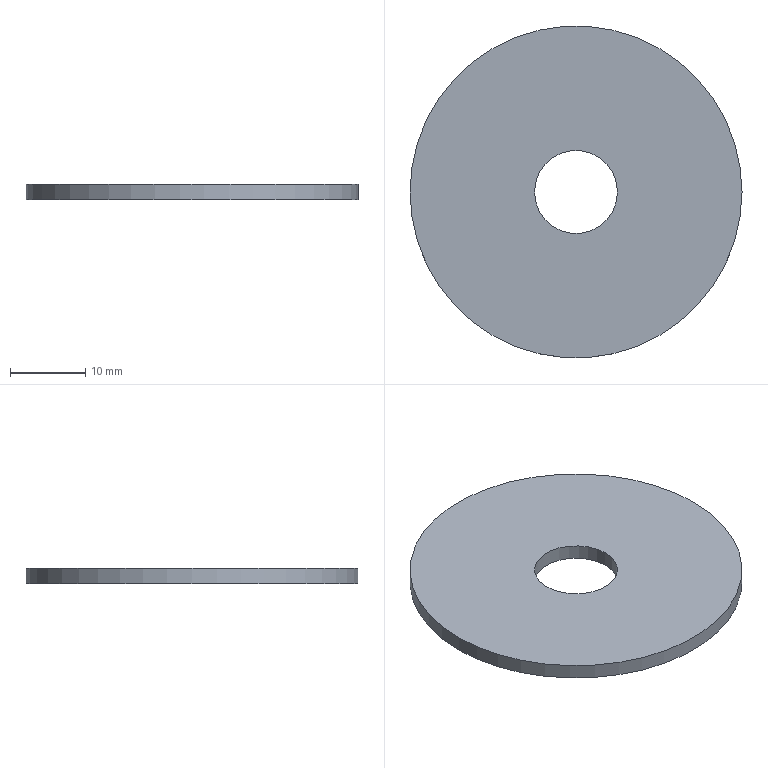Part | NX | features CYLINDER 1, DATUM_CSYS 1, HOLE PACKAGE 1, SIMPLE HOLE 1 | 1 solid | 4 faces | box 44 x 44 x 2 mm | volume 2851 mm3 | plane 2 | cylinder 2 | commonest cylinder face diameters 11 x1 44 x1
STEP:
#1=CARTESIAN_POINT('',(5.5,0.,2.));
#2=VERTEX_POINT('',#1);
#3=CARTESIAN_POINT('',(0.,0.,2.));
#4=DIRECTION('',(0.,0.,1.));
#5=DIRECTION('',(1.,0.,0.));
#6=AXIS2_PLACEMENT_3D('',#3,#4,#5);
#7=CIRCLE('',#6,5.5);
#8=EDGE_CURVE('',#2,#2,#7,.T.);
#9=ORIENTED_EDGE('',*,*,#8,.F.);
#10=EDGE_LOOP('',(#9));
#11=FACE_BOUND('',#10,.T.);
#12=CARTESIAN_POINT('',(-22.,0.,2.));
#13=VERTEX_POINT('',#12);
#14=CARTESIAN_POINT('',(0.,0.,2.));
#15=DIRECTION('',(0.,0.,-1.));
#16=DIRECTION('',(-1.,0.,0.));
#17=AXIS2_PLACEMENT_3D('',#14,#15,#16);
#18=CIRCLE('',#17,22.);
#19=EDGE_CURVE('',#13,#13,#18,.T.);
#20=ORIENTED_EDGE('',*,*,#19,.F.);
#21=EDGE_LOOP('',(#20));
#22=FACE_BOUND('',#21,.T.);
#23=CARTESIAN_POINT('',(0.,0.,2.));
#24=DIRECTION('',(0.,0.,1.));
#25=DIRECTION('',(1.,0.,0.));
#26=AXIS2_PLACEMENT_3D('',#23,#24,#25);
#27=PLANE('',#26);
#28=ADVANCED_FACE('',(#11,#22),#27,.T.);
#29=CARTESIAN_POINT('',(5.5,0.,0.));
#30=VERTEX_POINT('',#29);
#31=CARTESIAN_POINT('',(0.,0.,0.));
#32=DIRECTION('',(0.,0.,1.));
#33=DIRECTION('',(1.,0.,0.));
#34=AXIS2_PLACEMENT_3D('',#31,#32,#33);
#35=CIRCLE('',#34,5.5);
#36=EDGE_CURVE('',#30,#30,#35,.T.);
#37=ORIENTED_EDGE('',*,*,#36,.T.);
#38=EDGE_LOOP('',(#37));
#39=FACE_BOUND('',#38,.T.);
#40=CARTESIAN_POINT('',(22.,0.,0.));
#41=VERTEX_POINT('',#40);
#42=CARTESIAN_POINT('',(0.,0.,0.));
#43=DIRECTION('',(0.,0.,1.));
#44=DIRECTION('',(1.,0.,0.));
#45=AXIS2_PLACEMENT_3D('',#42,#43,#44);
#46=CIRCLE('',#45,22.);
#47=EDGE_CURVE('',#41,#41,#46,.T.);
#48=ORIENTED_EDGE('',*,*,#47,.F.);
#49=EDGE_LOOP('',(#48));
#50=FACE_BOUND('',#49,.T.);
#51=CARTESIAN_POINT('',(0.,0.,0.));
#52=DIRECTION('',(0.,0.,-1.));
#53=DIRECTION('',(-1.,0.,0.));
#54=AXIS2_PLACEMENT_3D('',#51,#52,#53);
#55=PLANE('',#54);
#56=ADVANCED_FACE('',(#39,#50),#55,.T.);
#57=ORIENTED_EDGE('',*,*,#19,.T.);
#58=EDGE_LOOP('',(#57));
#59=FACE_BOUND('',#58,.T.);
#60=ORIENTED_EDGE('',*,*,#47,.T.);
#61=EDGE_LOOP('',(#60));
#62=FACE_BOUND('',#61,.T.);
#63=CARTESIAN_POINT('',(0.,0.,0.));
#64=DIRECTION('',(0.,0.,1.));
#65=DIRECTION('',(1.,0.,0.));
#66=AXIS2_PLACEMENT_3D('',#63,#64,#65);
#67=CYLINDRICAL_SURFACE('',#66,22.);
#68=ADVANCED_FACE('',(#59,#62),#67,.T.);
#69=ORIENTED_EDGE('',*,*,#8,.T.);
#70=EDGE_LOOP('',(#69));
#71=FACE_BOUND('',#70,.T.);
#72=ORIENTED_EDGE('',*,*,#36,.F.);
#73=EDGE_LOOP('',(#72));
#74=FACE_BOUND('',#73,.T.);
#75=CARTESIAN_POINT('',(0.,0.,0.));
#76=DIRECTION('',(0.,0.,1.));
#77=DIRECTION('',(1.,0.,0.));
#78=AXIS2_PLACEMENT_3D('',#75,#76,#77);
#79=CYLINDRICAL_SURFACE('',#78,5.5);
#80=ADVANCED_FACE('',(#71,#74),#79,.F.);
#81=CLOSED_SHELL('',(#28,#56,#68,#80));
#82=MANIFOLD_SOLID_BREP('',#81);
#83=(LENGTH_UNIT()NAMED_UNIT(*)SI_UNIT(.MILLI.,.METRE.));
#84=UNCERTAINTY_MEASURE_WITH_UNIT(LENGTH_MEASURE(0.00001),#83,'','');
#85=(NAMED_UNIT(*)PLANE_ANGLE_UNIT()SI_UNIT($,.RADIAN.));
#86=(NAMED_UNIT(*)SI_UNIT($,.STERADIAN.)SOLID_ANGLE_UNIT());
#87=(GEOMETRIC_REPRESENTATION_CONTEXT(3)GLOBAL_UNCERTAINTY_ASSIGNED_CONTEXT((#84))GLOBAL_UNIT_ASSIGNED_CONTEXT((#83,#85,#86))REPRESENTATION_CONTEXT('',''));
#88=ADVANCED_BREP_SHAPE_REPRESENTATION('',(#82),#87);